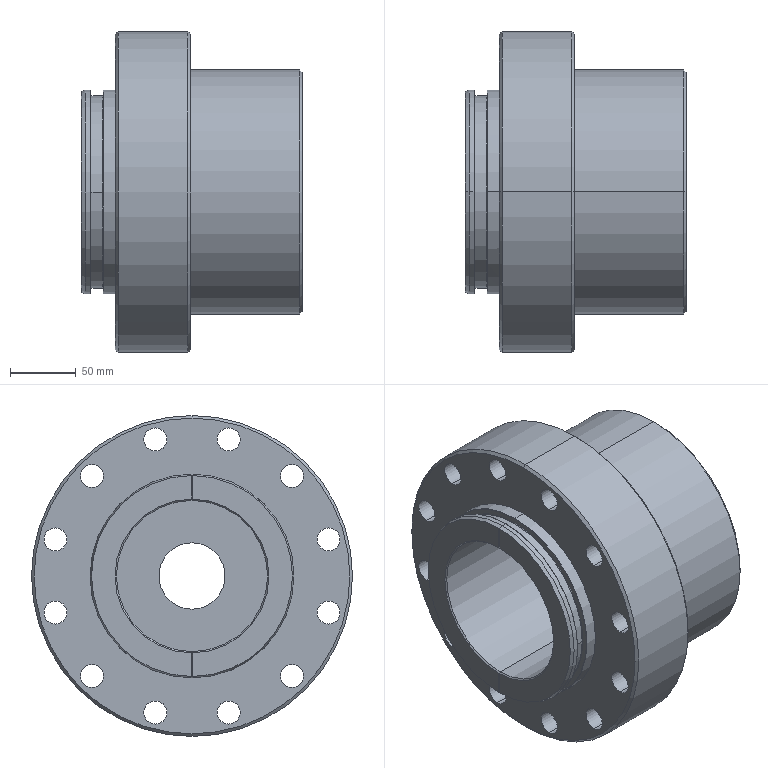Part | SolidWorks | features ICE 6, Chamfer 3, Cavity 2, Extrusion 1, HoleWzd 1 | 1 solid | 94 faces | box 168.5 x 244 x 244 mm | volume 4079273 mm3 | cylinder 50 | plane 22 | torus 12 | cone 10 | commonest cylinder face diameters 17.5 x24 50.5 x6 155 x4 54 x2 58 x2 60 x2